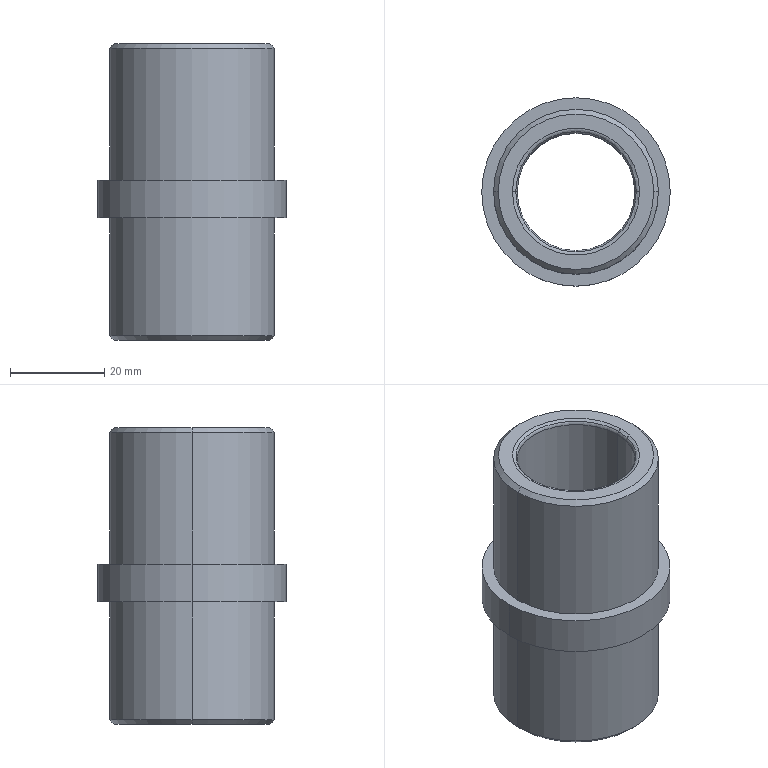Part | Creo | 1 solid | 24 faces | box 40 x 40 x 63 mm | volume 31902 mm3 | torus 8 | cylinder 8 | plane 4 | cone 4 | commonest cylinder face diameters 35 x4 25 x2 40 x2
STEP:
#1=CARTESIAN_POINT('',(143.5,-266.,-294.5));
#2=VERTEX_POINT('',#1);
#3=CARTESIAN_POINT('',(176.5,-266.,-294.5));
#4=VERTEX_POINT('',#3);
#5=CARTESIAN_POINT('',(160.,-266.,-294.5));
#6=DIRECTION('',(0.,0.,-1.));
#7=DIRECTION('',(-1.,0.,0.));
#8=AXIS2_PLACEMENT_3D('',#5,#6,#7);
#9=CIRCLE('',#8,16.5);
#10=EDGE_CURVE('',#2,#4,#9,.T.);
#11=ORIENTED_EDGE('',*,*,#10,.F.);
#12=CARTESIAN_POINT('',(160.,-266.,-294.5));
#13=DIRECTION('',(0.,0.,-1.));
#14=DIRECTION('',(1.,0.,0.));
#15=AXIS2_PLACEMENT_3D('',#12,#13,#14);
#16=CIRCLE('',#15,16.5);
#17=EDGE_CURVE('',#4,#2,#16,.T.);
#18=ORIENTED_EDGE('',*,*,#17,.F.);
#19=EDGE_LOOP('',(#11,#18));
#20=FACE_OUTER_BOUND('',#19,.F.);
#21=CARTESIAN_POINT('',(146.5,-266.,-294.5));
#22=VERTEX_POINT('',#21);
#23=CARTESIAN_POINT('',(173.5,-266.,-294.5));
#24=VERTEX_POINT('',#23);
#25=CARTESIAN_POINT('',(160.,-266.,-294.5));
#26=DIRECTION('',(0.,0.,1.));
#27=DIRECTION('',(-1.,0.,0.));
#28=AXIS2_PLACEMENT_3D('',#25,#26,#27);
#29=CIRCLE('',#28,13.5);
#30=EDGE_CURVE('',#22,#24,#29,.T.);
#31=ORIENTED_EDGE('',*,*,#30,.F.);
#32=CARTESIAN_POINT('',(160.,-266.,-294.5));
#33=DIRECTION('',(0.,0.,1.));
#34=DIRECTION('',(1.,0.,0.));
#35=AXIS2_PLACEMENT_3D('',#32,#33,#34);
#36=CIRCLE('',#35,13.5);
#37=EDGE_CURVE('',#24,#22,#36,.T.);
#38=ORIENTED_EDGE('',*,*,#37,.F.);
#39=EDGE_LOOP('',(#31,#38));
#40=FACE_BOUND('',#39,.F.);
#41=CARTESIAN_POINT('',(160.,-266.,-294.5));
#42=DIRECTION('',(0.,0.,-1.));
#43=DIRECTION('',(-1.,0.,0.));
#44=AXIS2_PLACEMENT_3D('',#41,#42,#43);
#45=PLANE('',#44);
#46=ADVANCED_FACE('',(#20,#40),#45,.T.);
#47=ORIENTED_EDGE('',*,*,#30,.T.);
#48=CARTESIAN_POINT('',(172.793,-266.,-294.207));
#49=VERTEX_POINT('',#48);
#50=CARTESIAN_POINT('',(173.5,-266.,-293.5));
#51=DIRECTION('',(0.,1.,0.));
#52=DIRECTION('',(0.,0.,-1.));
#53=AXIS2_PLACEMENT_3D('',#50,#51,#52);
#54=CIRCLE('',#53,1.);
#55=EDGE_CURVE('',#24,#49,#54,.T.);
#56=ORIENTED_EDGE('',*,*,#55,.T.);
#57=CARTESIAN_POINT('',(147.207,-266.,-294.207));
#58=VERTEX_POINT('',#57);
#59=CARTESIAN_POINT('',(160.,-266.,-294.207));
#60=DIRECTION('',(0.,0.,-1.));
#61=DIRECTION('',(1.,0.,0.));
#62=AXIS2_PLACEMENT_3D('',#59,#60,#61);
#63=CIRCLE('',#62,12.793);
#64=EDGE_CURVE('',#49,#58,#63,.T.);
#65=ORIENTED_EDGE('',*,*,#64,.T.);
#66=CARTESIAN_POINT('',(146.5,-266.,-293.5));
#67=DIRECTION('',(0.,-1.,0.));
#68=DIRECTION('',(0.,0.,-1.));
#69=AXIS2_PLACEMENT_3D('',#66,#67,#68);
#70=CIRCLE('',#69,1.);
#71=EDGE_CURVE('',#22,#58,#70,.T.);
#72=ORIENTED_EDGE('',*,*,#71,.F.);
#73=EDGE_LOOP('',(#47,#56,#65,#72));
#74=FACE_OUTER_BOUND('',#73,.F.);
#75=CARTESIAN_POINT('',(160.,-266.,-293.5));
#76=DIRECTION('',(0.,0.,-1.));
#77=DIRECTION('',(-1.,0.,0.));
#78=AXIS2_PLACEMENT_3D('',#75,#76,#77);
#79=TOROIDAL_SURFACE('',#78,13.5,1.);
#80=ADVANCED_FACE('',(#74),#79,.T.);
#81=ORIENTED_EDGE('',*,*,#37,.T.);
#82=ORIENTED_EDGE('',*,*,#71,.T.);
#83=CARTESIAN_POINT('',(160.,-266.,-294.207));
#84=DIRECTION('',(0.,0.,-1.));
#85=DIRECTION('',(-1.,0.,0.));
#86=AXIS2_PLACEMENT_3D('',#83,#84,#85);
#87=CIRCLE('',#86,12.793);
#88=EDGE_CURVE('',#58,#49,#87,.T.);
#89=ORIENTED_EDGE('',*,*,#88,.T.);
#90=ORIENTED_EDGE('',*,*,#55,.F.);
#91=EDGE_LOOP('',(#81,#82,#89,#90));
#92=FACE_OUTER_BOUND('',#91,.F.);
#93=CARTESIAN_POINT('',(160.,-266.,-293.5));
#94=DIRECTION('',(0.,0.,-1.));
#95=DIRECTION('',(-1.,0.,0.));
#96=AXIS2_PLACEMENT_3D('',#93,#94,#95);
#97=TOROIDAL_SURFACE('',#96,13.5,1.);
#98=ADVANCED_FACE('',(#92),#97,.T.);
#99=CARTESIAN_POINT('',(172.5,-266.,-293.5));
#100=VERTEX_POINT('',#99);
#101=CARTESIAN_POINT('',(147.5,-266.,-293.5));
#102=VERTEX_POINT('',#101);
#103=CARTESIAN_POINT('',(160.,-266.,-293.5));
#104=DIRECTION('',(0.,0.,1.));
#105=DIRECTION('',(1.,0.,0.));
#106=AXIS2_PLACEMENT_3D('',#103,#104,#105);
#107=CIRCLE('',#106,12.5);
#108=EDGE_CURVE('',#100,#102,#107,.T.);
#109=ORIENTED_EDGE('',*,*,#108,.F.);
#110=CARTESIAN_POINT('',(173.5,-266.,-293.5));
#111=DIRECTION('',(0.,1.,0.));
#112=DIRECTION('',(-0.7071,0.,-0.7071));
#113=AXIS2_PLACEMENT_3D('',#110,#111,#112);
#114=CIRCLE('',#113,1.);
#115=EDGE_CURVE('',#49,#100,#114,.T.);
#116=ORIENTED_EDGE('',*,*,#115,.F.);
#117=ORIENTED_EDGE('',*,*,#88,.F.);
#118=CARTESIAN_POINT('',(146.5,-266.,-293.5));
#119=DIRECTION('',(0.,-1.,0.));
#120=DIRECTION('',(0.7071,0.,-0.7071));
#121=AXIS2_PLACEMENT_3D('',#118,#119,#120);
#122=CIRCLE('',#121,1.);
#123=EDGE_CURVE('',#58,#102,#122,.T.);
#124=ORIENTED_EDGE('',*,*,#123,.T.);
#125=EDGE_LOOP('',(#109,#116,#117,#124));
#126=FACE_OUTER_BOUND('',#125,.F.);
#127=CARTESIAN_POINT('',(160.,-266.,-293.5));
#128=DIRECTION('',(0.,0.,-1.));
#129=DIRECTION('',(-1.,0.,0.));
#130=AXIS2_PLACEMENT_3D('',#127,#128,#129);
#131=TOROIDAL_SURFACE('',#130,13.5,1.);
#132=ADVANCED_FACE('',(#126),#131,.T.);
#133=ORIENTED_EDGE('',*,*,#108,.T.);
#134=CARTESIAN_POINT('',(147.5,-266.,-232.5));
#135=VERTEX_POINT('',#134);
#136=CARTESIAN_POINT('',(147.5,-266.,-293.5));
#137=DIRECTION('',(0.,0.,1.));
#138=VECTOR('',#137,61.);
#139=LINE('',#136,#138);
#140=EDGE_CURVE('',#102,#135,#139,.T.);
#141=ORIENTED_EDGE('',*,*,#140,.T.);
#142=CARTESIAN_POINT('',(172.5,-266.,-232.5));
#143=VERTEX_POINT('',#142);
#144=CARTESIAN_POINT('',(160.,-266.,-232.5));
#145=DIRECTION('',(0.,0.,-1.));
#146=DIRECTION('',(-1.,0.,0.));
#147=AXIS2_PLACEMENT_3D('',#144,#145,#146);
#148=CIRCLE('',#147,12.5);
#149=EDGE_CURVE('',#135,#143,#148,.T.);
#150=ORIENTED_EDGE('',*,*,#149,.T.);
#151=CARTESIAN_POINT('',(172.5,-266.,-293.5));
#152=DIRECTION('',(0.,0.,1.));
#153=VECTOR('',#152,61.);
#154=LINE('',#151,#153);
#155=EDGE_CURVE('',#100,#143,#154,.T.);
#156=ORIENTED_EDGE('',*,*,#155,.F.);
#157=EDGE_LOOP('',(#133,#141,#150,#156));
#158=FACE_OUTER_BOUND('',#157,.F.);
#159=CARTESIAN_POINT('',(160.,-266.,-284.5));
#160=DIRECTION('',(0.,0.,1.));
#161=DIRECTION('',(1.,0.,0.));
#162=AXIS2_PLACEMENT_3D('',#159,#160,#161);
#163=CYLINDRICAL_SURFACE('',#162,12.5);
#164=ADVANCED_FACE('',(#158),#163,.F.);
#165=CARTESIAN_POINT('',(160.,-266.,-293.5));
#166=DIRECTION('',(0.,0.,1.));
#167=DIRECTION('',(-1.,0.,0.));
#168=AXIS2_PLACEMENT_3D('',#165,#166,#167);
#169=CIRCLE('',#168,12.5);
#170=EDGE_CURVE('',#102,#100,#169,.T.);
#171=ORIENTED_EDGE('',*,*,#170,.T.);
#172=ORIENTED_EDGE('',*,*,#155,.T.);
#173=CARTESIAN_POINT('',(160.,-266.,-232.5));
#174=DIRECTION('',(0.,0.,-1.));
#175=DIRECTION('',(1.,0.,0.));
#176=AXIS2_PLACEMENT_3D('',#173,#174,#175);
#177=CIRCLE('',#176,12.5);
#178=EDGE_CURVE('',#143,#135,#177,.T.);
#179=ORIENTED_EDGE('',*,*,#178,.T.);
#180=ORIENTED_EDGE('',*,*,#140,.F.);
#181=EDGE_LOOP('',(#171,#172,#179,#180));
#182=FACE_OUTER_BOUND('',#181,.F.);
#183=CARTESIAN_POINT('',(160.,-266.,-284.5));
#184=DIRECTION('',(0.,0.,1.));
#185=DIRECTION('',(1.,0.,0.));
#186=AXIS2_PLACEMENT_3D('',#183,#184,#185);
#187=CYLINDRICAL_SURFACE('',#186,12.5);
#188=ADVANCED_FACE('',(#182),#187,.F.);
#189=ORIENTED_EDGE('',*,*,#170,.F.);
#190=ORIENTED_EDGE('',*,*,#123,.F.);
#191=ORIENTED_EDGE('',*,*,#64,.F.);
#192=ORIENTED_EDGE('',*,*,#115,.T.);
#193=EDGE_LOOP('',(#189,#190,#191,#192));
#194=FACE_OUTER_BOUND('',#193,.F.);
#195=CARTESIAN_POINT('',(160.,-266.,-293.5));
#196=DIRECTION('',(0.,0.,-1.));
#197=DIRECTION('',(-1.,0.,0.));
#198=AXIS2_PLACEMENT_3D('',#195,#196,#197);
#199=TOROIDAL_SURFACE('',#198,13.5,1.);
#200=ADVANCED_FACE('',(#194),#199,.T.);
#201=ORIENTED_EDGE('',*,*,#178,.F.);
#202=CARTESIAN_POINT('',(172.793,-266.,-231.793));
#203=VERTEX_POINT('',#202);
#204=CARTESIAN_POINT('',(173.5,-266.,-232.5));
#205=DIRECTION('',(0.,-1.,0.));
#206=DIRECTION('',(-0.7071,0.,0.7071));
#207=AXIS2_PLACEMENT_3D('',#204,#205,#206);
#208=CIRCLE('',#207,1.);
#209=EDGE_CURVE('',#203,#143,#208,.T.);
#210=ORIENTED_EDGE('',*,*,#209,.F.);
#211=CARTESIAN_POINT('',(147.207,-266.,-231.793));
#212=VERTEX_POINT('',#211);
#213=CARTESIAN_POINT('',(160.,-266.,-231.793));
#214=DIRECTION('',(0.,0.,1.));
#215=DIRECTION('',(-1.,0.,0.));
#216=AXIS2_PLACEMENT_3D('',#213,#214,#215);
#217=CIRCLE('',#216,12.793);
#218=EDGE_CURVE('',#212,#203,#217,.T.);
#219=ORIENTED_EDGE('',*,*,#218,.F.);
#220=CARTESIAN_POINT('',(146.5,-266.,-232.5));
#221=DIRECTION('',(0.,1.,0.));
#222=DIRECTION('',(0.7071,0.,0.7071));
#223=AXIS2_PLACEMENT_3D('',#220,#221,#222);
#224=CIRCLE('',#223,1.);
#225=EDGE_CURVE('',#212,#135,#224,.T.);
#226=ORIENTED_EDGE('',*,*,#225,.T.);
#227=EDGE_LOOP('',(#201,#210,#219,#226));
#228=FACE_OUTER_BOUND('',#227,.F.);
#229=CARTESIAN_POINT('',(160.,-266.,-232.5));
#230=DIRECTION('',(0.,0.,1.));
#231=DIRECTION('',(1.,0.,0.));
#232=AXIS2_PLACEMENT_3D('',#229,#230,#231);
#233=TOROIDAL_SURFACE('',#232,13.5,1.);
#234=ADVANCED_FACE('',(#228),#233,.T.);
#235=ORIENTED_EDGE('',*,*,#149,.F.);
#236=ORIENTED_EDGE('',*,*,#225,.F.);
#237=CARTESIAN_POINT('',(160.,-266.,-231.793));
#238=DIRECTION('',(0.,0.,1.));
#239=DIRECTION('',(1.,0.,0.));
#240=AXIS2_PLACEMENT_3D('',#237,#238,#239);
#241=CIRCLE('',#240,12.793);
#242=EDGE_CURVE('',#203,#212,#241,.T.);
#243=ORIENTED_EDGE('',*,*,#242,.F.);
#244=ORIENTED_EDGE('',*,*,#209,.T.);
#245=EDGE_LOOP('',(#235,#236,#243,#244));
#246=FACE_OUTER_BOUND('',#245,.F.);
#247=CARTESIAN_POINT('',(160.,-266.,-232.5));
#248=DIRECTION('',(0.,0.,1.));
#249=DIRECTION('',(1.,0.,0.));
#250=AXIS2_PLACEMENT_3D('',#247,#248,#249);
#251=TOROIDAL_SURFACE('',#250,13.5,1.);
#252=ADVANCED_FACE('',(#246),#251,.T.);
#253=CARTESIAN_POINT('',(146.5,-266.,-231.5));
#254=VERTEX_POINT('',#253);
#255=CARTESIAN_POINT('',(173.5,-266.,-231.5));
#256=VERTEX_POINT('',#255);
#257=CARTESIAN_POINT('',(160.,-266.,-231.5));
#258=DIRECTION('',(0.,0.,-1.));
#259=DIRECTION('',(-1.,0.,0.));
#260=AXIS2_PLACEMENT_3D('',#257,#258,#259);
#261=CIRCLE('',#260,13.5);
#262=EDGE_CURVE('',#254,#256,#261,.T.);
#263=ORIENTED_EDGE('',*,*,#262,.T.);
#264=CARTESIAN_POINT('',(173.5,-266.,-232.5));
#265=DIRECTION('',(0.,-1.,0.));
#266=DIRECTION('',(0.,0.,1.));
#267=AXIS2_PLACEMENT_3D('',#264,#265,#266);
#268=CIRCLE('',#267,1.);
#269=EDGE_CURVE('',#256,#203,#268,.T.);
#270=ORIENTED_EDGE('',*,*,#269,.T.);
#271=ORIENTED_EDGE('',*,*,#242,.T.);
#272=CARTESIAN_POINT('',(146.5,-266.,-232.5));
#273=DIRECTION('',(0.,1.,0.));
#274=DIRECTION('',(0.,0.,1.));
#275=AXIS2_PLACEMENT_3D('',#272,#273,#274);
#276=CIRCLE('',#275,1.);
#277=EDGE_CURVE('',#254,#212,#276,.T.);
#278=ORIENTED_EDGE('',*,*,#277,.F.);
#279=EDGE_LOOP('',(#263,#270,#271,#278));
#280=FACE_OUTER_BOUND('',#279,.F.);
#281=CARTESIAN_POINT('',(160.,-266.,-232.5));
#282=DIRECTION('',(0.,0.,1.));
#283=DIRECTION('',(1.,0.,0.));
#284=AXIS2_PLACEMENT_3D('',#281,#282,#283);
#285=TOROIDAL_SURFACE('',#284,13.5,1.);
#286=ADVANCED_FACE('',(#280),#285,.T.);
#287=CARTESIAN_POINT('',(176.5,-266.,-231.5));
#288=VERTEX_POINT('',#287);
#289=CARTESIAN_POINT('',(143.5,-266.,-231.5));
#290=VERTEX_POINT('',#289);
#291=CARTESIAN_POINT('',(160.,-266.,-231.5));
#292=DIRECTION('',(0.,0.,1.));
#293=DIRECTION('',(1.,0.,0.));
#294=AXIS2_PLACEMENT_3D('',#291,#292,#293);
#295=CIRCLE('',#294,16.5);
#296=EDGE_CURVE('',#288,#290,#295,.T.);
#297=ORIENTED_EDGE('',*,*,#296,.F.);
#298=CARTESIAN_POINT('',(160.,-266.,-231.5));
#299=DIRECTION('',(0.,0.,1.));
#300=DIRECTION('',(-1.,0.,0.));
#301=AXIS2_PLACEMENT_3D('',#298,#299,#300);
#302=CIRCLE('',#301,16.5);
#303=EDGE_CURVE('',#290,#288,#302,.T.);
#304=ORIENTED_EDGE('',*,*,#303,.F.);
#305=EDGE_LOOP('',(#297,#304));
#306=FACE_OUTER_BOUND('',#305,.F.);
#307=CARTESIAN_POINT('',(160.,-266.,-231.5));
#308=DIRECTION('',(0.,0.,-1.));
#309=DIRECTION('',(1.,0.,0.));
#310=AXIS2_PLACEMENT_3D('',#307,#308,#309);
#311=CIRCLE('',#310,13.5);
#312=EDGE_CURVE('',#256,#254,#311,.T.);
#313=ORIENTED_EDGE('',*,*,#312,.F.);
#314=ORIENTED_EDGE('',*,*,#262,.F.);
#315=EDGE_LOOP('',(#313,#314));
#316=FACE_BOUND('',#315,.F.);
#317=CARTESIAN_POINT('',(160.,-266.,-231.5));
#318=DIRECTION('',(0.,0.,1.));
#319=DIRECTION('',(1.,0.,0.));
#320=AXIS2_PLACEMENT_3D('',#317,#318,#319);
#321=PLANE('',#320);
#322=ADVANCED_FACE('',(#306,#316),#321,.T.);
#323=ORIENTED_EDGE('',*,*,#312,.T.);
#324=ORIENTED_EDGE('',*,*,#277,.T.);
#325=ORIENTED_EDGE('',*,*,#218,.T.);
#326=ORIENTED_EDGE('',*,*,#269,.F.);
#327=EDGE_LOOP('',(#323,#324,#325,#326));
#328=FACE_OUTER_BOUND('',#327,.F.);
#329=CARTESIAN_POINT('',(160.,-266.,-232.5));
#330=DIRECTION('',(0.,0.,1.));
#331=DIRECTION('',(1.,0.,0.));
#332=AXIS2_PLACEMENT_3D('',#329,#330,#331);
#333=TOROIDAL_SURFACE('',#332,13.5,1.);
#334=ADVANCED_FACE('',(#328),#333,.T.);
#335=ORIENTED_EDGE('',*,*,#296,.T.);
#336=CARTESIAN_POINT('',(142.5,-266.,-232.5));
#337=VERTEX_POINT('',#336);
#338=CARTESIAN_POINT('',(143.5,-266.,-231.5));
#339=DIRECTION('',(-0.7071,0.,-0.7071));
#340=VECTOR('',#339,1.414);
#341=LINE('',#338,#340);
#342=EDGE_CURVE('',#290,#337,#341,.T.);
#343=ORIENTED_EDGE('',*,*,#342,.T.);
#344=CARTESIAN_POINT('',(177.5,-266.,-232.5));
#345=VERTEX_POINT('',#344);
#346=CARTESIAN_POINT('',(160.,-266.,-232.5));
#347=DIRECTION('',(0.,0.,1.));
#348=DIRECTION('',(1.,0.,0.));
#349=AXIS2_PLACEMENT_3D('',#346,#347,#348);
#350=CIRCLE('',#349,17.5);
#351=EDGE_CURVE('',#345,#337,#350,.T.);
#352=ORIENTED_EDGE('',*,*,#351,.F.);
#353=CARTESIAN_POINT('',(176.5,-266.,-231.5));
#354=DIRECTION('',(0.7071,0.,-0.7071));
#355=VECTOR('',#354,1.414);
#356=LINE('',#353,#355);
#357=EDGE_CURVE('',#288,#345,#356,.T.);
#358=ORIENTED_EDGE('',*,*,#357,.F.);
#359=EDGE_LOOP('',(#335,#343,#352,#358));
#360=FACE_OUTER_BOUND('',#359,.F.);
#361=CARTESIAN_POINT('',(160.,-266.,-232.));
#362=DIRECTION('',(0.,0.,-1.));
#363=DIRECTION('',(-1.,0.,0.));
#364=AXIS2_PLACEMENT_3D('',#361,#362,#363);
#365=CONICAL_SURFACE('',#364,17.,45.);
#366=ADVANCED_FACE('',(#360),#365,.T.);
#367=ORIENTED_EDGE('',*,*,#303,.T.);
#368=ORIENTED_EDGE('',*,*,#357,.T.);
#369=CARTESIAN_POINT('',(160.,-266.,-232.5));
#370=DIRECTION('',(0.,0.,1.));
#371=DIRECTION('',(-1.,0.,0.));
#372=AXIS2_PLACEMENT_3D('',#369,#370,#371);
#373=CIRCLE('',#372,17.5);
#374=EDGE_CURVE('',#337,#345,#373,.T.);
#375=ORIENTED_EDGE('',*,*,#374,.F.);
#376=ORIENTED_EDGE('',*,*,#342,.F.);
#377=EDGE_LOOP('',(#367,#368,#375,#376));
#378=FACE_OUTER_BOUND('',#377,.F.);
#379=CARTESIAN_POINT('',(160.,-266.,-232.));
#380=DIRECTION('',(0.,0.,-1.));
#381=DIRECTION('',(-1.,0.,0.));
#382=AXIS2_PLACEMENT_3D('',#379,#380,#381);
#383=CONICAL_SURFACE('',#382,17.,45.);
#384=ADVANCED_FACE('',(#378),#383,.T.);
#385=CARTESIAN_POINT('',(177.5,-266.,-260.5));
#386=VERTEX_POINT('',#385);
#387=CARTESIAN_POINT('',(142.5,-266.,-260.5));
#388=VERTEX_POINT('',#387);
#389=CARTESIAN_POINT('',(160.,-266.,-260.5));
#390=DIRECTION('',(0.,0.,-1.));
#391=DIRECTION('',(1.,0.,0.));
#392=AXIS2_PLACEMENT_3D('',#389,#390,#391);
#393=CIRCLE('',#392,17.5);
#394=EDGE_CURVE('',#386,#388,#393,.T.);
#395=ORIENTED_EDGE('',*,*,#394,.T.);
#396=CARTESIAN_POINT('',(142.5,-266.,-260.5));
#397=DIRECTION('',(0.,0.,1.));
#398=VECTOR('',#397,28.);
#399=LINE('',#396,#398);
#400=EDGE_CURVE('',#388,#337,#399,.T.);
#401=ORIENTED_EDGE('',*,*,#400,.T.);
#402=ORIENTED_EDGE('',*,*,#374,.T.);
#403=CARTESIAN_POINT('',(177.5,-266.,-260.5));
#404=DIRECTION('',(0.,0.,1.));
#405=VECTOR('',#404,28.);
#406=LINE('',#403,#405);
#407=EDGE_CURVE('',#386,#345,#406,.T.);
#408=ORIENTED_EDGE('',*,*,#407,.F.);
#409=EDGE_LOOP('',(#395,#401,#402,#408));
#410=FACE_OUTER_BOUND('',#409,.F.);
#411=CARTESIAN_POINT('',(160.,-266.,-284.5));
#412=DIRECTION('',(0.,0.,1.));
#413=DIRECTION('',(1.,0.,0.));
#414=AXIS2_PLACEMENT_3D('',#411,#412,#413);
#415=CYLINDRICAL_SURFACE('',#414,17.5);
#416=ADVANCED_FACE('',(#410),#415,.T.);
#417=CARTESIAN_POINT('',(140.,-266.,-260.5));
#418=VERTEX_POINT('',#417);
#419=CARTESIAN_POINT('',(180.,-266.,-260.5));
#420=VERTEX_POINT('',#419);
#421=CARTESIAN_POINT('',(160.,-266.,-260.5));
#422=DIRECTION('',(0.,0.,1.));
#423=DIRECTION('',(-1.,0.,0.));
#424=AXIS2_PLACEMENT_3D('',#421,#422,#423);
#425=CIRCLE('',#424,20.);
#426=EDGE_CURVE('',#418,#420,#425,.T.);
#427=ORIENTED_EDGE('',*,*,#426,.F.);
#428=CARTESIAN_POINT('',(160.,-266.,-260.5));
#429=DIRECTION('',(0.,0.,1.));
#430=DIRECTION('',(1.,0.,0.));
#431=AXIS2_PLACEMENT_3D('',#428,#429,#430);
#432=CIRCLE('',#431,20.);
#433=EDGE_CURVE('',#420,#418,#432,.T.);
#434=ORIENTED_EDGE('',*,*,#433,.F.);
#435=EDGE_LOOP('',(#427,#434));
#436=FACE_OUTER_BOUND('',#435,.F.);
#437=ORIENTED_EDGE('',*,*,#394,.F.);
#438=CARTESIAN_POINT('',(160.,-266.,-260.5));
#439=DIRECTION('',(0.,0.,-1.));
#440=DIRECTION('',(-1.,0.,0.));
#441=AXIS2_PLACEMENT_3D('',#438,#439,#440);
#442=CIRCLE('',#441,17.5);
#443=EDGE_CURVE('',#388,#386,#442,.T.);
#444=ORIENTED_EDGE('',*,*,#443,.F.);
#445=EDGE_LOOP('',(#437,#444));
#446=FACE_BOUND('',#445,.F.);
#447=CARTESIAN_POINT('',(160.,-266.,-260.5));
#448=DIRECTION('',(0.,0.,1.));
#449=DIRECTION('',(1.,0.,0.));
#450=AXIS2_PLACEMENT_3D('',#447,#448,#449);
#451=PLANE('',#450);
#452=ADVANCED_FACE('',(#436,#446),#451,.T.);
#453=ORIENTED_EDGE('',*,*,#443,.T.);
#454=ORIENTED_EDGE('',*,*,#407,.T.);
#455=ORIENTED_EDGE('',*,*,#351,.T.);
#456=ORIENTED_EDGE('',*,*,#400,.F.);
#457=EDGE_LOOP('',(#453,#454,#455,#456));
#458=FACE_OUTER_BOUND('',#457,.F.);
#459=CARTESIAN_POINT('',(160.,-266.,-284.5));
#460=DIRECTION('',(0.,0.,1.));
#461=DIRECTION('',(1.,0.,0.));
#462=AXIS2_PLACEMENT_3D('',#459,#460,#461);
#463=CYLINDRICAL_SURFACE('',#462,17.5);
#464=ADVANCED_FACE('',(#458),#463,.T.);
#465=CARTESIAN_POINT('',(180.,-266.,-268.5));
#466=VERTEX_POINT('',#465);
#467=CARTESIAN_POINT('',(140.,-266.,-268.5));
#468=VERTEX_POINT('',#467);
#469=CARTESIAN_POINT('',(160.,-266.,-268.5));
#470=DIRECTION('',(0.,0.,-1.));
#471=DIRECTION('',(1.,0.,0.));
#472=AXIS2_PLACEMENT_3D('',#469,#470,#471);
#473=CIRCLE('',#472,20.);
#474=EDGE_CURVE('',#466,#468,#473,.T.);
#475=ORIENTED_EDGE('',*,*,#474,.T.);
#476=CARTESIAN_POINT('',(140.,-266.,-260.5));
#477=DIRECTION('',(0.,0.,-1.));
#478=VECTOR('',#477,8.);
#479=LINE('',#476,#478);
#480=EDGE_CURVE('',#418,#468,#479,.T.);
#481=ORIENTED_EDGE('',*,*,#480,.F.);
#482=ORIENTED_EDGE('',*,*,#426,.T.);
#483=CARTESIAN_POINT('',(180.,-266.,-260.5));
#484=DIRECTION('',(0.,0.,-1.));
#485=VECTOR('',#484,8.);
#486=LINE('',#483,#485);
#487=EDGE_CURVE('',#420,#466,#486,.T.);
#488=ORIENTED_EDGE('',*,*,#487,.T.);
#489=EDGE_LOOP('',(#475,#481,#482,#488));
#490=FACE_OUTER_BOUND('',#489,.F.);
#491=CARTESIAN_POINT('',(160.,-266.,-260.5));
#492=DIRECTION('',(0.,0.,-1.));
#493=DIRECTION('',(-1.,0.,0.));
#494=AXIS2_PLACEMENT_3D('',#491,#492,#493);
#495=CYLINDRICAL_SURFACE('',#494,20.);
#496=ADVANCED_FACE('',(#490),#495,.T.);
#497=ORIENTED_EDGE('',*,*,#474,.F.);
#498=CARTESIAN_POINT('',(160.,-266.,-268.5));
#499=DIRECTION('',(0.,0.,-1.));
#500=DIRECTION('',(-1.,0.,0.));
#501=AXIS2_PLACEMENT_3D('',#498,#499,#500);
#502=CIRCLE('',#501,20.);
#503=EDGE_CURVE('',#468,#466,#502,.T.);
#504=ORIENTED_EDGE('',*,*,#503,.F.);
#505=EDGE_LOOP('',(#497,#504));
#506=FACE_OUTER_BOUND('',#505,.F.);
#507=CARTESIAN_POINT('',(142.5,-266.,-268.5));
#508=VERTEX_POINT('',#507);
#509=CARTESIAN_POINT('',(177.5,-266.,-268.5));
#510=VERTEX_POINT('',#509);
#511=CARTESIAN_POINT('',(160.,-266.,-268.5));
#512=DIRECTION('',(0.,0.,1.));
#513=DIRECTION('',(-1.,0.,0.));
#514=AXIS2_PLACEMENT_3D('',#511,#512,#513);
#515=CIRCLE('',#514,17.5);
#516=EDGE_CURVE('',#508,#510,#515,.T.);
#517=ORIENTED_EDGE('',*,*,#516,.F.);
#518=CARTESIAN_POINT('',(160.,-266.,-268.5));
#519=DIRECTION('',(0.,0.,1.));
#520=DIRECTION('',(1.,0.,0.));
#521=AXIS2_PLACEMENT_3D('',#518,#519,#520);
#522=CIRCLE('',#521,17.5);
#523=EDGE_CURVE('',#510,#508,#522,.T.);
#524=ORIENTED_EDGE('',*,*,#523,.F.);
#525=EDGE_LOOP('',(#517,#524));
#526=FACE_BOUND('',#525,.F.);
#527=CARTESIAN_POINT('',(160.,-266.,-268.5));
#528=DIRECTION('',(0.,0.,-1.));
#529=DIRECTION('',(-1.,0.,0.));
#530=AXIS2_PLACEMENT_3D('',#527,#528,#529);
#531=PLANE('',#530);
#532=ADVANCED_FACE('',(#506,#526),#531,.T.);
#533=ORIENTED_EDGE('',*,*,#516,.T.);
#534=CARTESIAN_POINT('',(177.5,-266.,-293.5));
#535=VERTEX_POINT('',#534);
#536=CARTESIAN_POINT('',(177.5,-266.,-293.5));
#537=DIRECTION('',(0.,0.,1.));
#538=VECTOR('',#537,25.);
#539=LINE('',#536,#538);
#540=EDGE_CURVE('',#535,#510,#539,.T.);
#541=ORIENTED_EDGE('',*,*,#540,.F.);
#542=CARTESIAN_POINT('',(142.5,-266.,-293.5));
#543=VERTEX_POINT('',#542);
#544=CARTESIAN_POINT('',(160.,-266.,-293.5));
#545=DIRECTION('',(0.,0.,-1.));
#546=DIRECTION('',(1.,0.,0.));
#547=AXIS2_PLACEMENT_3D('',#544,#545,#546);
#548=CIRCLE('',#547,17.5);
#549=EDGE_CURVE('',#535,#543,#548,.T.);
#550=ORIENTED_EDGE('',*,*,#549,.T.);
#551=CARTESIAN_POINT('',(142.5,-266.,-293.5));
#552=DIRECTION('',(0.,0.,1.));
#553=VECTOR('',#552,25.);
#554=LINE('',#551,#553);
#555=EDGE_CURVE('',#543,#508,#554,.T.);
#556=ORIENTED_EDGE('',*,*,#555,.T.);
#557=EDGE_LOOP('',(#533,#541,#550,#556));
#558=FACE_OUTER_BOUND('',#557,.F.);
#559=CARTESIAN_POINT('',(160.,-266.,-294.5));
#560=DIRECTION('',(0.,0.,1.));
#561=DIRECTION('',(1.,0.,0.));
#562=AXIS2_PLACEMENT_3D('',#559,#560,#561);
#563=CYLINDRICAL_SURFACE('',#562,17.5);
#564=ADVANCED_FACE('',(#558),#563,.T.);
#565=ORIENTED_EDGE('',*,*,#523,.T.);
#566=ORIENTED_EDGE('',*,*,#555,.F.);
#567=CARTESIAN_POINT('',(160.,-266.,-293.5));
#568=DIRECTION('',(0.,0.,-1.));
#569=DIRECTION('',(-1.,0.,0.));
#570=AXIS2_PLACEMENT_3D('',#567,#568,#569);
#571=CIRCLE('',#570,17.5);
#572=EDGE_CURVE('',#543,#535,#571,.T.);
#573=ORIENTED_EDGE('',*,*,#572,.T.);
#574=ORIENTED_EDGE('',*,*,#540,.T.);
#575=EDGE_LOOP('',(#565,#566,#573,#574));
#576=FACE_OUTER_BOUND('',#575,.F.);
#577=CARTESIAN_POINT('',(160.,-266.,-294.5));
#578=DIRECTION('',(0.,0.,1.));
#579=DIRECTION('',(1.,0.,0.));
#580=AXIS2_PLACEMENT_3D('',#577,#578,#579);
#581=CYLINDRICAL_SURFACE('',#580,17.5);
#582=ADVANCED_FACE('',(#576),#581,.T.);
#583=ORIENTED_EDGE('',*,*,#10,.T.);
#584=CARTESIAN_POINT('',(176.5,-266.,-294.5));
#585=DIRECTION('',(0.7071,0.,0.7071));
#586=VECTOR('',#585,1.414);
#587=LINE('',#584,#586);
#588=EDGE_CURVE('',#4,#535,#587,.T.);
#589=ORIENTED_EDGE('',*,*,#588,.T.);
#590=ORIENTED_EDGE('',*,*,#572,.F.);
#591=CARTESIAN_POINT('',(143.5,-266.,-294.5));
#592=DIRECTION('',(-0.7071,0.,0.7071));
#593=VECTOR('',#592,1.414);
#594=LINE('',#591,#593);
#595=EDGE_CURVE('',#2,#543,#594,.T.);
#596=ORIENTED_EDGE('',*,*,#595,.F.);
#597=EDGE_LOOP('',(#583,#589,#590,#596));
#598=FACE_OUTER_BOUND('',#597,.F.);
#599=CARTESIAN_POINT('',(160.,-266.,-294.));
#600=DIRECTION('',(0.,0.,1.));
#601=DIRECTION('',(1.,0.,0.));
#602=AXIS2_PLACEMENT_3D('',#599,#600,#601);
#603=CONICAL_SURFACE('',#602,17.,45.);
#604=ADVANCED_FACE('',(#598),#603,.T.);
#605=ORIENTED_EDGE('',*,*,#17,.T.);
#606=ORIENTED_EDGE('',*,*,#595,.T.);
#607=ORIENTED_EDGE('',*,*,#549,.F.);
#608=ORIENTED_EDGE('',*,*,#588,.F.);
#609=EDGE_LOOP('',(#605,#606,#607,#608));
#610=FACE_OUTER_BOUND('',#609,.F.);
#611=CARTESIAN_POINT('',(160.,-266.,-294.));
#612=DIRECTION('',(0.,0.,1.));
#613=DIRECTION('',(1.,0.,0.));
#614=AXIS2_PLACEMENT_3D('',#611,#612,#613);
#615=CONICAL_SURFACE('',#614,17.,45.);
#616=ADVANCED_FACE('',(#610),#615,.T.);
#617=ORIENTED_EDGE('',*,*,#503,.T.);
#618=ORIENTED_EDGE('',*,*,#487,.F.);
#619=ORIENTED_EDGE('',*,*,#433,.T.);
#620=ORIENTED_EDGE('',*,*,#480,.T.);
#621=EDGE_LOOP('',(#617,#618,#619,#620));
#622=FACE_OUTER_BOUND('',#621,.F.);
#623=CARTESIAN_POINT('',(160.,-266.,-260.5));
#624=DIRECTION('',(0.,0.,-1.));
#625=DIRECTION('',(-1.,0.,0.));
#626=AXIS2_PLACEMENT_3D('',#623,#624,#625);
#627=CYLINDRICAL_SURFACE('',#626,20.);
#628=ADVANCED_FACE('',(#622),#627,.T.);
#629=CLOSED_SHELL('',(#46,#80,#98,#132,#164,#188,#200,#234,#252,#286,#322,#334,#366,#384,#416,#452,#464,#496,#532,#564,#582,#604,#616,#628));
#630=MANIFOLD_SOLID_BREP('',#629);
#631=(LENGTH_UNIT()NAMED_UNIT(*)SI_UNIT(.MILLI.,.METRE.));
#632=UNCERTAINTY_MEASURE_WITH_UNIT(LENGTH_MEASURE(0.008468),#631,'','');
#633=(NAMED_UNIT(*)PLANE_ANGLE_UNIT()SI_UNIT($,.RADIAN.));
#634=PLANE_ANGLE_MEASURE_WITH_UNIT(PLANE_ANGLE_MEASURE(0.01745),#633);
#635=(CONVERSION_BASED_UNIT('DEGREE',#634)NAMED_UNIT(*)PLANE_ANGLE_UNIT());
#636=(NAMED_UNIT(*)SI_UNIT($,.STERADIAN.)SOLID_ANGLE_UNIT());
#637=(GEOMETRIC_REPRESENTATION_CONTEXT(3)GLOBAL_UNCERTAINTY_ASSIGNED_CONTEXT((#632))GLOBAL_UNIT_ASSIGNED_CONTEXT((#631,#635,#636))REPRESENTATION_CONTEXT('',''));
#638=ADVANCED_BREP_SHAPE_REPRESENTATION('',(#630),#637);